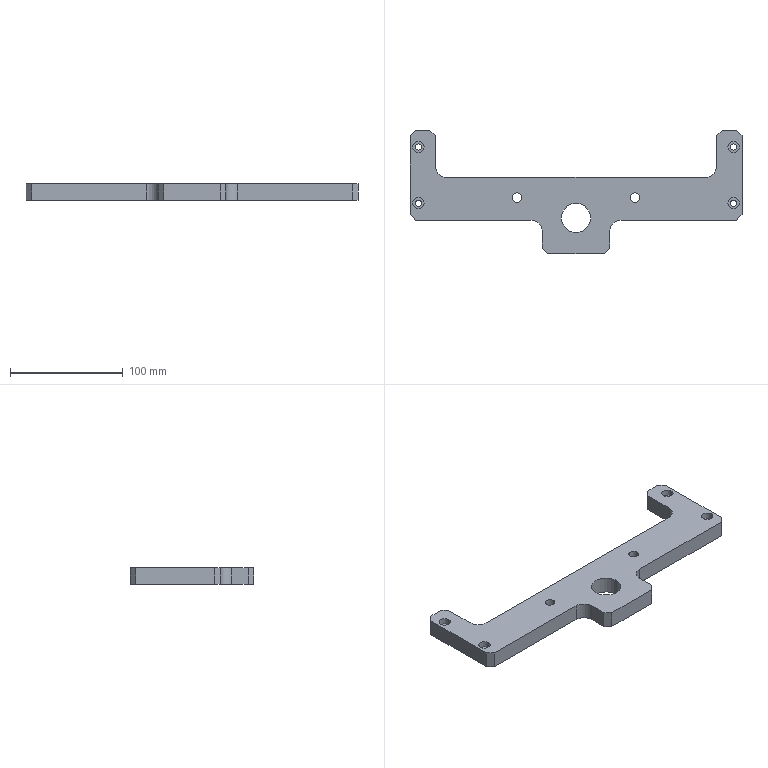Part | STEP file | Polisher mounting plate | 1 solid | 52 faces | box 295 x 110 x 15 mm | volume 210947 mm3 | cylinder 26 | plane 26 | commonest cylinder face diameters 5.5 x8 10 x8 8.5 x4 20 x4 26 x2